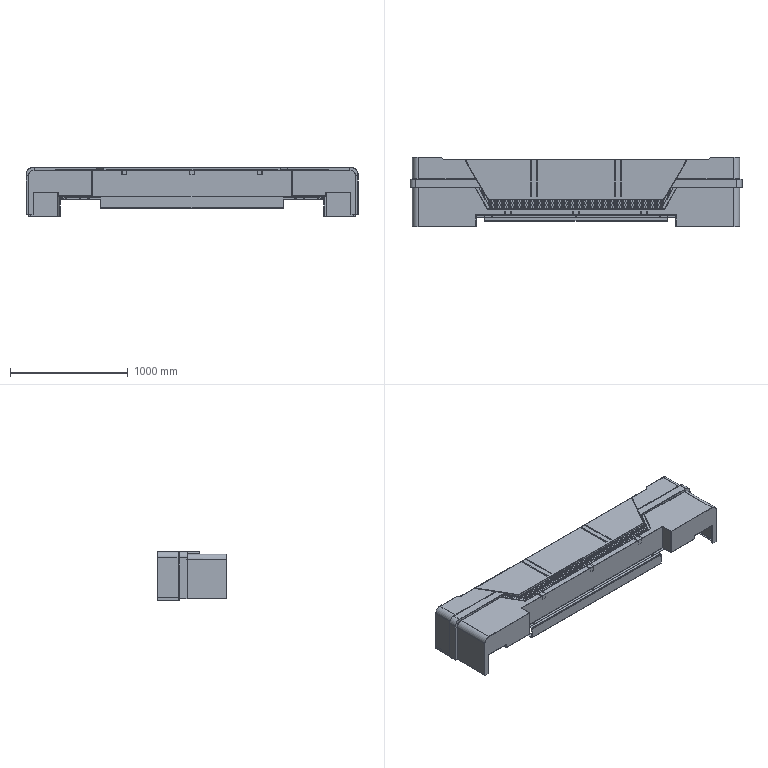Part | SolidWorks | features ReferencePattern 2, MirrorCompFeat 1 | 39 solids | 4101 faces | volume 9484925 mm3 | cylinder 2452 | plane 1560 | spline 89 | commonest cylinder face diameters 7.2 x1908 6 x100 6.4 x90 4 x89 1 x83 2 x58